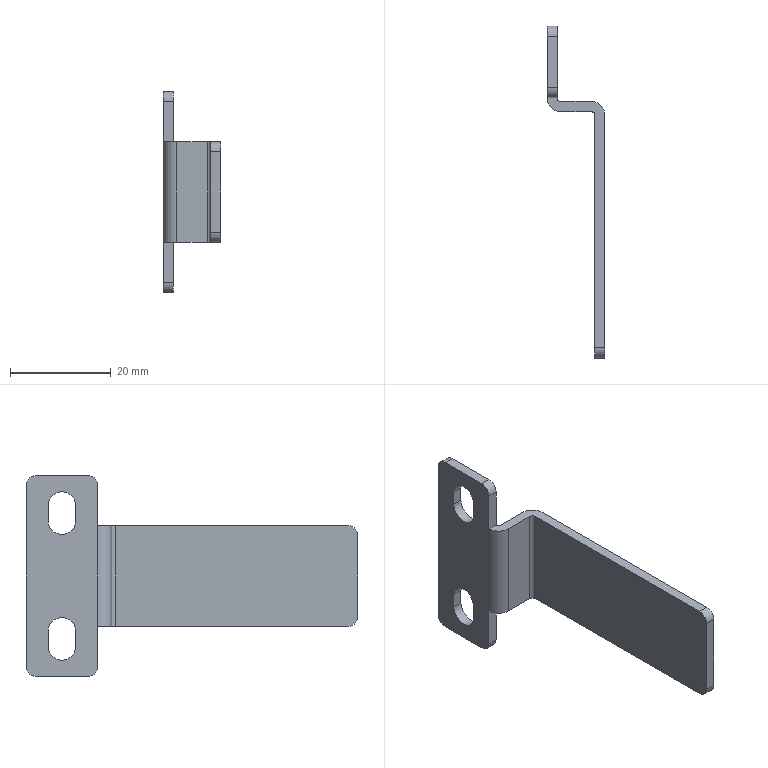Part | STEP file | 1 solid | 32 faces | box 11.5 x 66 x 40 mm | volume 3360 mm3 | plane 18 | cylinder 14 | commonest cylinder face diameters 4 x6 5.5 x4 1.473 x2 5.473 x2